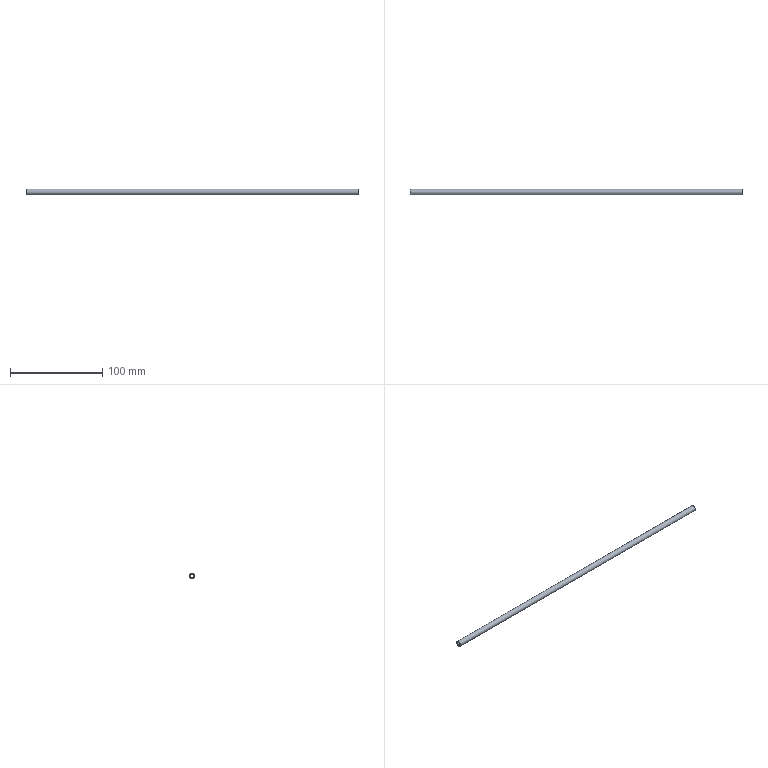Part | NX | features solid 2 | 1 solid | 4 faces | box 360 x 6 x 6 mm | volume 5655 mm3 | cylinder 2 | plane 2 | commonest cylinder face diameters 4 x1 6 x1
STEP:
#1=CARTESIAN_POINT('',(470.,-66.,347.));
#2=VERTEX_POINT('',#1);
#3=CARTESIAN_POINT('',(470.,-64.,347.));
#4=DIRECTION('',(-1.,0.,0.));
#5=DIRECTION('',(0.,-1.,0.));
#6=AXIS2_PLACEMENT_3D('',#3,#4,#5);
#7=CIRCLE('',#6,2.);
#8=EDGE_CURVE('',#2,#2,#7,.T.);
#9=ORIENTED_EDGE('',*,*,#8,.F.);
#10=EDGE_LOOP('',(#9));
#11=FACE_BOUND('',#10,.T.);
#12=CARTESIAN_POINT('',(110.,-66.,347.));
#13=VERTEX_POINT('',#12);
#14=CARTESIAN_POINT('',(110.,-64.,347.));
#15=DIRECTION('',(-1.,0.,0.));
#16=DIRECTION('',(0.,-1.,0.));
#17=AXIS2_PLACEMENT_3D('',#14,#15,#16);
#18=CIRCLE('',#17,2.);
#19=EDGE_CURVE('',#13,#13,#18,.T.);
#20=ORIENTED_EDGE('',*,*,#19,.T.);
#21=EDGE_LOOP('',(#20));
#22=FACE_BOUND('',#21,.T.);
#23=CARTESIAN_POINT('',(241.176,-64.,347.));
#24=DIRECTION('',(1.,0.,0.));
#25=DIRECTION('',(0.,1.,0.));
#26=AXIS2_PLACEMENT_3D('',#23,#24,#25);
#27=CYLINDRICAL_SURFACE('',#26,2.);
#28=ADVANCED_FACE('',(#11,#22),#27,.F.);
#29=CARTESIAN_POINT('',(470.,-67.,347.));
#30=VERTEX_POINT('',#29);
#31=CARTESIAN_POINT('',(470.,-64.,347.));
#32=DIRECTION('',(-1.,0.,0.));
#33=DIRECTION('',(0.,-1.,0.));
#34=AXIS2_PLACEMENT_3D('',#31,#32,#33);
#35=CIRCLE('',#34,3.);
#36=EDGE_CURVE('',#30,#30,#35,.T.);
#37=ORIENTED_EDGE('',*,*,#36,.T.);
#38=EDGE_LOOP('',(#37));
#39=FACE_BOUND('',#38,.T.);
#40=CARTESIAN_POINT('',(110.,-67.,347.));
#41=VERTEX_POINT('',#40);
#42=CARTESIAN_POINT('',(110.,-64.,347.));
#43=DIRECTION('',(-1.,0.,0.));
#44=DIRECTION('',(0.,-1.,0.));
#45=AXIS2_PLACEMENT_3D('',#42,#43,#44);
#46=CIRCLE('',#45,3.);
#47=EDGE_CURVE('',#41,#41,#46,.T.);
#48=ORIENTED_EDGE('',*,*,#47,.F.);
#49=EDGE_LOOP('',(#48));
#50=FACE_BOUND('',#49,.T.);
#51=CARTESIAN_POINT('',(241.176,-64.,347.));
#52=DIRECTION('',(1.,0.,0.));
#53=DIRECTION('',(0.,1.,0.));
#54=AXIS2_PLACEMENT_3D('',#51,#52,#53);
#55=CYLINDRICAL_SURFACE('',#54,3.);
#56=ADVANCED_FACE('',(#39,#50),#55,.T.);
#57=ORIENTED_EDGE('',*,*,#8,.T.);
#58=EDGE_LOOP('',(#57));
#59=FACE_BOUND('',#58,.T.);
#60=ORIENTED_EDGE('',*,*,#36,.F.);
#61=EDGE_LOOP('',(#60));
#62=FACE_BOUND('',#61,.T.);
#63=CARTESIAN_POINT('',(470.,-64.,347.));
#64=DIRECTION('',(-1.,0.,0.));
#65=DIRECTION('',(0.,-1.,0.));
#66=AXIS2_PLACEMENT_3D('',#63,#64,#65);
#67=PLANE('',#66);
#68=ADVANCED_FACE('',(#59,#62),#67,.F.);
#69=ORIENTED_EDGE('',*,*,#19,.F.);
#70=EDGE_LOOP('',(#69));
#71=FACE_BOUND('',#70,.T.);
#72=ORIENTED_EDGE('',*,*,#47,.T.);
#73=EDGE_LOOP('',(#72));
#74=FACE_BOUND('',#73,.T.);
#75=CARTESIAN_POINT('',(110.,35.,347.));
#76=DIRECTION('',(-1.,0.,0.));
#77=DIRECTION('',(0.,-1.,0.));
#78=AXIS2_PLACEMENT_3D('',#75,#76,#77);
#79=PLANE('',#78);
#80=ADVANCED_FACE('',(#71,#74),#79,.T.);
#81=CLOSED_SHELL('',(#28,#56,#68,#80));
#82=MANIFOLD_SOLID_BREP('',#81);
#83=(LENGTH_UNIT()NAMED_UNIT(*)SI_UNIT(.MILLI.,.METRE.));
#84=UNCERTAINTY_MEASURE_WITH_UNIT(LENGTH_MEASURE(0.00001),#83,'','');
#85=(NAMED_UNIT(*)PLANE_ANGLE_UNIT()SI_UNIT($,.RADIAN.));
#86=(NAMED_UNIT(*)SI_UNIT($,.STERADIAN.)SOLID_ANGLE_UNIT());
#87=(GEOMETRIC_REPRESENTATION_CONTEXT(3)GLOBAL_UNCERTAINTY_ASSIGNED_CONTEXT((#84))GLOBAL_UNIT_ASSIGNED_CONTEXT((#83,#85,#86))REPRESENTATION_CONTEXT('',''));
#88=ADVANCED_BREP_SHAPE_REPRESENTATION('',(#82),#87);